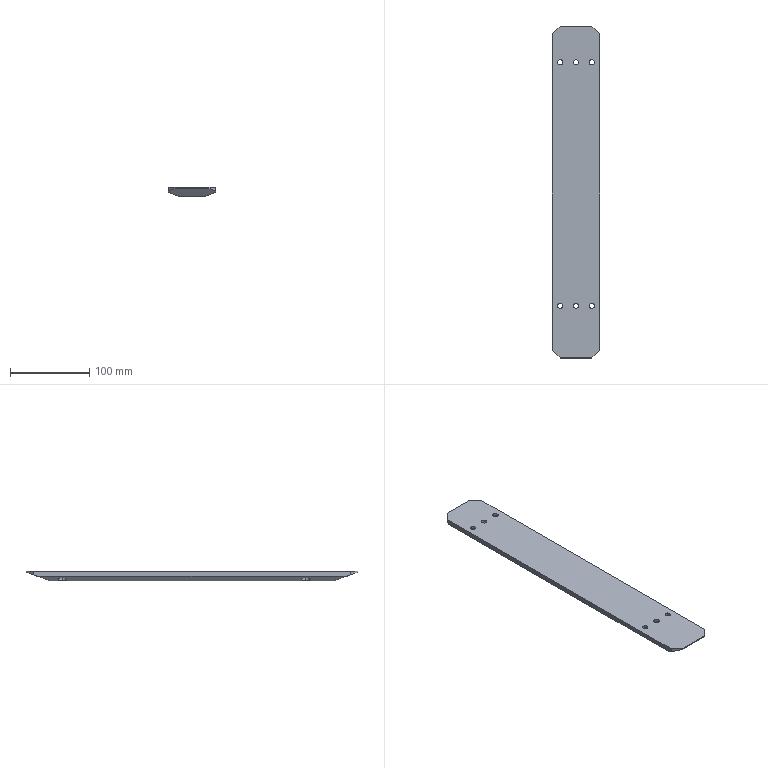Part | SolidWorks | features BaseBody 1 | 1 solid | 44 faces | box 60 x 420 x 12 mm | volume 246931 mm3 | cylinder 24 | plane 20 | commonest cylinder face diameters 6.6 x12 11 x12
STEP:
#1=CARTESIAN_POINT('',(25.5,164.,9.));
#2=VERTEX_POINT('',#1);
#3=CARTESIAN_POINT('',(14.5,164.,9.));
#4=VERTEX_POINT('',#3);
#5=CARTESIAN_POINT('',(20.,164.,9.));
#6=DIRECTION('',(0.,0.,-1.));
#7=DIRECTION('',(-1.,0.,0.));
#8=AXIS2_PLACEMENT_3D('',#5,#6,#7);
#9=CIRCLE('',#8,5.5);
#10=EDGE_CURVE('',#2,#4,#9,.T.);
#11=ORIENTED_EDGE('',*,*,#10,.F.);
#12=CARTESIAN_POINT('',(25.5,164.,3.822));
#13=VERTEX_POINT('',#12);
#14=CARTESIAN_POINT('',(25.5,164.,0.));
#15=DIRECTION('',(0.,0.,-1.));
#16=VECTOR('',#15,1000.);
#17=LINE('',#14,#16);
#18=EDGE_CURVE('',#2,#13,#17,.T.);
#19=ORIENTED_EDGE('',*,*,#18,.T.);
#20=CARTESIAN_POINT('',(15.,161.709,0.));
#21=VERTEX_POINT('',#20);
#22=CARTESIAN_POINT('',(25.5,164.,3.822));
#23=CARTESIAN_POINT('',(25.5,156.466,3.822));
#24=CARTESIAN_POINT('',(18.139,154.859,1.142));
#25=CARTESIAN_POINT('',(15.,161.709,0.));
#26=(BOUNDED_CURVE()B_SPLINE_CURVE(3,(#22,#23,#24,#25),.UNSPECIFIED.,.F.,.F.)B_SPLINE_CURVE_WITH_KNOTS((4,4),(3.142,5.853),.UNSPECIFIED.)CURVE()GEOMETRIC_REPRESENTATION_ITEM()RATIONAL_B_SPLINE_CURVE((1.,0.4755,0.4755,1.))REPRESENTATION_ITEM(''));
#27=EDGE_CURVE('',#13,#21,#26,.T.);
#28=ORIENTED_EDGE('',*,*,#27,.T.);
#29=CARTESIAN_POINT('',(14.5,164.,0.));
#30=VERTEX_POINT('',#29);
#31=CARTESIAN_POINT('',(20.,164.,0.));
#32=DIRECTION('',(0.,0.,-1.));
#33=DIRECTION('',(-1.,0.,0.));
#34=AXIS2_PLACEMENT_3D('',#31,#32,#33);
#35=CIRCLE('',#34,5.5);
#36=EDGE_CURVE('',#21,#30,#35,.T.);
#37=ORIENTED_EDGE('',*,*,#36,.T.);
#38=CARTESIAN_POINT('',(14.5,164.,0.));
#39=DIRECTION('',(0.,0.,-1.));
#40=VECTOR('',#39,1000.);
#41=LINE('',#38,#40);
#42=EDGE_CURVE('',#4,#30,#41,.T.);
#43=ORIENTED_EDGE('',*,*,#42,.F.);
#44=EDGE_LOOP('',(#11,#19,#28,#37,#43));
#45=FACE_OUTER_BOUND('',#44,.T.);
#46=CARTESIAN_POINT('',(20.,164.,0.));
#47=DIRECTION('',(0.,0.,-1.));
#48=DIRECTION('',(-1.,0.,0.));
#49=AXIS2_PLACEMENT_3D('',#46,#47,#48);
#50=CYLINDRICAL_SURFACE('',#49,5.5);
#51=ADVANCED_FACE('',(#45),#50,.F.);
#52=CARTESIAN_POINT('',(23.3,164.,12.));
#53=VERTEX_POINT('',#52);
#54=CARTESIAN_POINT('',(16.7,164.,12.));
#55=VERTEX_POINT('',#54);
#56=CARTESIAN_POINT('',(20.,164.,12.));
#57=DIRECTION('',(0.,0.,-1.));
#58=DIRECTION('',(-1.,0.,0.));
#59=AXIS2_PLACEMENT_3D('',#56,#57,#58);
#60=CIRCLE('',#59,3.3);
#61=EDGE_CURVE('',#53,#55,#60,.T.);
#62=ORIENTED_EDGE('',*,*,#61,.F.);
#63=CARTESIAN_POINT('',(23.3,164.,9.));
#64=VERTEX_POINT('',#63);
#65=CARTESIAN_POINT('',(23.3,164.,0.));
#66=DIRECTION('',(0.,0.,-1.));
#67=VECTOR('',#66,1000.);
#68=LINE('',#65,#67);
#69=EDGE_CURVE('',#53,#64,#68,.T.);
#70=ORIENTED_EDGE('',*,*,#69,.T.);
#71=CARTESIAN_POINT('',(16.7,164.,9.));
#72=VERTEX_POINT('',#71);
#73=CARTESIAN_POINT('',(20.,164.,9.));
#74=DIRECTION('',(0.,0.,-1.));
#75=DIRECTION('',(-1.,0.,0.));
#76=AXIS2_PLACEMENT_3D('',#73,#74,#75);
#77=CIRCLE('',#76,3.3);
#78=EDGE_CURVE('',#64,#72,#77,.T.);
#79=ORIENTED_EDGE('',*,*,#78,.T.);
#80=CARTESIAN_POINT('',(16.7,164.,0.));
#81=DIRECTION('',(0.,0.,-1.));
#82=VECTOR('',#81,1000.);
#83=LINE('',#80,#82);
#84=EDGE_CURVE('',#55,#72,#83,.T.);
#85=ORIENTED_EDGE('',*,*,#84,.F.);
#86=EDGE_LOOP('',(#62,#70,#79,#85));
#87=FACE_OUTER_BOUND('',#86,.T.);
#88=CARTESIAN_POINT('',(20.,164.,0.));
#89=DIRECTION('',(0.,0.,-1.));
#90=DIRECTION('',(-1.,0.,0.));
#91=AXIS2_PLACEMENT_3D('',#88,#89,#90);
#92=CYLINDRICAL_SURFACE('',#91,3.3);
#93=ADVANCED_FACE('',(#87),#92,.F.);
#94=CARTESIAN_POINT('',(5.5,164.,9.));
#95=VERTEX_POINT('',#94);
#96=CARTESIAN_POINT('',(-5.5,164.,9.));
#97=VERTEX_POINT('',#96);
#98=CARTESIAN_POINT('',(0.,164.,9.));
#99=DIRECTION('',(0.,0.,-1.));
#100=DIRECTION('',(-1.,0.,0.));
#101=AXIS2_PLACEMENT_3D('',#98,#99,#100);
#102=CIRCLE('',#101,5.5);
#103=EDGE_CURVE('',#95,#97,#102,.T.);
#104=ORIENTED_EDGE('',*,*,#103,.F.);
#105=CARTESIAN_POINT('',(5.5,164.,0.));
#106=VERTEX_POINT('',#105);
#107=CARTESIAN_POINT('',(5.5,164.,0.));
#108=DIRECTION('',(0.,0.,-1.));
#109=VECTOR('',#108,1000.);
#110=LINE('',#107,#109);
#111=EDGE_CURVE('',#95,#106,#110,.T.);
#112=ORIENTED_EDGE('',*,*,#111,.T.);
#113=CARTESIAN_POINT('',(-5.5,164.,0.));
#114=VERTEX_POINT('',#113);
#115=CARTESIAN_POINT('',(0.,164.,0.));
#116=DIRECTION('',(0.,0.,-1.));
#117=DIRECTION('',(-1.,0.,0.));
#118=AXIS2_PLACEMENT_3D('',#115,#116,#117);
#119=CIRCLE('',#118,5.5);
#120=EDGE_CURVE('',#106,#114,#119,.T.);
#121=ORIENTED_EDGE('',*,*,#120,.T.);
#122=CARTESIAN_POINT('',(-5.5,164.,0.));
#123=DIRECTION('',(0.,0.,-1.));
#124=VECTOR('',#123,1000.);
#125=LINE('',#122,#124);
#126=EDGE_CURVE('',#97,#114,#125,.T.);
#127=ORIENTED_EDGE('',*,*,#126,.F.);
#128=EDGE_LOOP('',(#104,#112,#121,#127));
#129=FACE_OUTER_BOUND('',#128,.T.);
#130=CARTESIAN_POINT('',(0.,164.,0.));
#131=DIRECTION('',(0.,0.,-1.));
#132=DIRECTION('',(-1.,0.,0.));
#133=AXIS2_PLACEMENT_3D('',#130,#131,#132);
#134=CYLINDRICAL_SURFACE('',#133,5.5);
#135=ADVANCED_FACE('',(#129),#134,.F.);
#136=CARTESIAN_POINT('',(3.3,164.,12.));
#137=VERTEX_POINT('',#136);
#138=CARTESIAN_POINT('',(-3.3,164.,12.));
#139=VERTEX_POINT('',#138);
#140=CARTESIAN_POINT('',(0.,164.,12.));
#141=DIRECTION('',(0.,0.,-1.));
#142=DIRECTION('',(-1.,0.,0.));
#143=AXIS2_PLACEMENT_3D('',#140,#141,#142);
#144=CIRCLE('',#143,3.3);
#145=EDGE_CURVE('',#137,#139,#144,.T.);
#146=ORIENTED_EDGE('',*,*,#145,.F.);
#147=CARTESIAN_POINT('',(3.3,164.,9.));
#148=VERTEX_POINT('',#147);
#149=CARTESIAN_POINT('',(3.3,164.,0.));
#150=DIRECTION('',(0.,0.,-1.));
#151=VECTOR('',#150,1000.);
#152=LINE('',#149,#151);
#153=EDGE_CURVE('',#137,#148,#152,.T.);
#154=ORIENTED_EDGE('',*,*,#153,.T.);
#155=CARTESIAN_POINT('',(-3.3,164.,9.));
#156=VERTEX_POINT('',#155);
#157=CARTESIAN_POINT('',(0.,164.,9.));
#158=DIRECTION('',(0.,0.,-1.));
#159=DIRECTION('',(-1.,0.,0.));
#160=AXIS2_PLACEMENT_3D('',#157,#158,#159);
#161=CIRCLE('',#160,3.3);
#162=EDGE_CURVE('',#148,#156,#161,.T.);
#163=ORIENTED_EDGE('',*,*,#162,.T.);
#164=CARTESIAN_POINT('',(-3.3,164.,0.));
#165=DIRECTION('',(0.,0.,-1.));
#166=VECTOR('',#165,1000.);
#167=LINE('',#164,#166);
#168=EDGE_CURVE('',#139,#156,#167,.T.);
#169=ORIENTED_EDGE('',*,*,#168,.F.);
#170=EDGE_LOOP('',(#146,#154,#163,#169));
#171=FACE_OUTER_BOUND('',#170,.T.);
#172=CARTESIAN_POINT('',(0.,164.,0.));
#173=DIRECTION('',(0.,0.,-1.));
#174=DIRECTION('',(-1.,0.,0.));
#175=AXIS2_PLACEMENT_3D('',#172,#173,#174);
#176=CYLINDRICAL_SURFACE('',#175,3.3);
#177=ADVANCED_FACE('',(#171),#176,.F.);
#178=CARTESIAN_POINT('',(-14.5,164.,9.));
#179=VERTEX_POINT('',#178);
#180=CARTESIAN_POINT('',(-25.5,164.,9.));
#181=VERTEX_POINT('',#180);
#182=CARTESIAN_POINT('',(-20.,164.,9.));
#183=DIRECTION('',(0.,0.,-1.));
#184=DIRECTION('',(-1.,0.,0.));
#185=AXIS2_PLACEMENT_3D('',#182,#183,#184);
#186=CIRCLE('',#185,5.5);
#187=EDGE_CURVE('',#179,#181,#186,.T.);
#188=ORIENTED_EDGE('',*,*,#187,.F.);
#189=CARTESIAN_POINT('',(-14.5,164.,0.));
#190=VERTEX_POINT('',#189);
#191=CARTESIAN_POINT('',(-14.5,164.,0.));
#192=DIRECTION('',(0.,0.,-1.));
#193=VECTOR('',#192,1000.);
#194=LINE('',#191,#193);
#195=EDGE_CURVE('',#179,#190,#194,.T.);
#196=ORIENTED_EDGE('',*,*,#195,.T.);
#197=CARTESIAN_POINT('',(-15.,161.709,0.));
#198=VERTEX_POINT('',#197);
#199=CARTESIAN_POINT('',(-20.,164.,0.));
#200=DIRECTION('',(0.,0.,-1.));
#201=DIRECTION('',(-1.,0.,0.));
#202=AXIS2_PLACEMENT_3D('',#199,#200,#201);
#203=CIRCLE('',#202,5.5);
#204=EDGE_CURVE('',#190,#198,#203,.T.);
#205=ORIENTED_EDGE('',*,*,#204,.T.);
#206=CARTESIAN_POINT('',(-25.5,164.,3.822));
#207=VERTEX_POINT('',#206);
#208=CARTESIAN_POINT('',(-15.,161.709,0.));
#209=CARTESIAN_POINT('',(-18.139,154.859,1.142));
#210=CARTESIAN_POINT('',(-25.5,156.466,3.822));
#211=CARTESIAN_POINT('',(-25.5,164.,3.822));
#212=(BOUNDED_CURVE()B_SPLINE_CURVE(3,(#208,#209,#210,#211),.UNSPECIFIED.,.F.,.T.)B_SPLINE_CURVE_WITH_KNOTS((4,4),(0.4297,3.142),.UNSPECIFIED.)CURVE()GEOMETRIC_REPRESENTATION_ITEM()RATIONAL_B_SPLINE_CURVE((1.,0.4755,0.4755,1.))REPRESENTATION_ITEM(''));
#213=EDGE_CURVE('',#198,#207,#212,.T.);
#214=ORIENTED_EDGE('',*,*,#213,.T.);
#215=CARTESIAN_POINT('',(-25.5,164.,0.));
#216=DIRECTION('',(0.,0.,-1.));
#217=VECTOR('',#216,1000.);
#218=LINE('',#215,#217);
#219=EDGE_CURVE('',#181,#207,#218,.T.);
#220=ORIENTED_EDGE('',*,*,#219,.F.);
#221=EDGE_LOOP('',(#188,#196,#205,#214,#220));
#222=FACE_OUTER_BOUND('',#221,.T.);
#223=CARTESIAN_POINT('',(-20.,164.,0.));
#224=DIRECTION('',(0.,0.,-1.));
#225=DIRECTION('',(-1.,0.,0.));
#226=AXIS2_PLACEMENT_3D('',#223,#224,#225);
#227=CYLINDRICAL_SURFACE('',#226,5.5);
#228=ADVANCED_FACE('',(#222),#227,.F.);
#229=CARTESIAN_POINT('',(-16.7,164.,12.));
#230=VERTEX_POINT('',#229);
#231=CARTESIAN_POINT('',(-23.3,164.,12.));
#232=VERTEX_POINT('',#231);
#233=CARTESIAN_POINT('',(-20.,164.,12.));
#234=DIRECTION('',(0.,0.,-1.));
#235=DIRECTION('',(-1.,0.,0.));
#236=AXIS2_PLACEMENT_3D('',#233,#234,#235);
#237=CIRCLE('',#236,3.3);
#238=EDGE_CURVE('',#230,#232,#237,.T.);
#239=ORIENTED_EDGE('',*,*,#238,.F.);
#240=CARTESIAN_POINT('',(-16.7,164.,9.));
#241=VERTEX_POINT('',#240);
#242=CARTESIAN_POINT('',(-16.7,164.,0.));
#243=DIRECTION('',(0.,0.,-1.));
#244=VECTOR('',#243,1000.);
#245=LINE('',#242,#244);
#246=EDGE_CURVE('',#230,#241,#245,.T.);
#247=ORIENTED_EDGE('',*,*,#246,.T.);
#248=CARTESIAN_POINT('',(-23.3,164.,9.));
#249=VERTEX_POINT('',#248);
#250=CARTESIAN_POINT('',(-20.,164.,9.));
#251=DIRECTION('',(0.,0.,-1.));
#252=DIRECTION('',(-1.,0.,0.));
#253=AXIS2_PLACEMENT_3D('',#250,#251,#252);
#254=CIRCLE('',#253,3.3);
#255=EDGE_CURVE('',#241,#249,#254,.T.);
#256=ORIENTED_EDGE('',*,*,#255,.T.);
#257=CARTESIAN_POINT('',(-23.3,164.,0.));
#258=DIRECTION('',(0.,0.,-1.));
#259=VECTOR('',#258,1000.);
#260=LINE('',#257,#259);
#261=EDGE_CURVE('',#232,#249,#260,.T.);
#262=ORIENTED_EDGE('',*,*,#261,.F.);
#263=EDGE_LOOP('',(#239,#247,#256,#262));
#264=FACE_OUTER_BOUND('',#263,.T.);
#265=CARTESIAN_POINT('',(-20.,164.,0.));
#266=DIRECTION('',(0.,0.,-1.));
#267=DIRECTION('',(-1.,0.,0.));
#268=AXIS2_PLACEMENT_3D('',#265,#266,#267);
#269=CYLINDRICAL_SURFACE('',#268,3.3);
#270=ADVANCED_FACE('',(#264),#269,.F.);
#271=CARTESIAN_POINT('',(25.5,-144.,9.));
#272=VERTEX_POINT('',#271);
#273=CARTESIAN_POINT('',(14.5,-144.,9.));
#274=VERTEX_POINT('',#273);
#275=CARTESIAN_POINT('',(20.,-144.,9.));
#276=DIRECTION('',(0.,0.,-1.));
#277=DIRECTION('',(-1.,0.,0.));
#278=AXIS2_PLACEMENT_3D('',#275,#276,#277);
#279=CIRCLE('',#278,5.5);
#280=EDGE_CURVE('',#272,#274,#279,.T.);
#281=ORIENTED_EDGE('',*,*,#280,.F.);
#282=CARTESIAN_POINT('',(25.5,-144.,3.822));
#283=VERTEX_POINT('',#282);
#284=CARTESIAN_POINT('',(25.5,-144.,0.));
#285=DIRECTION('',(0.,0.,-1.));
#286=VECTOR('',#285,1000.);
#287=LINE('',#284,#286);
#288=EDGE_CURVE('',#272,#283,#287,.T.);
#289=ORIENTED_EDGE('',*,*,#288,.T.);
#290=CARTESIAN_POINT('',(15.,-146.291,0.));
#291=VERTEX_POINT('',#290);
#292=CARTESIAN_POINT('',(25.5,-144.,3.822));
#293=CARTESIAN_POINT('',(25.5,-151.534,3.822));
#294=CARTESIAN_POINT('',(18.139,-153.141,1.142));
#295=CARTESIAN_POINT('',(15.,-146.291,0.));
#296=(BOUNDED_CURVE()B_SPLINE_CURVE(3,(#292,#293,#294,#295),.UNSPECIFIED.,.F.,.F.)B_SPLINE_CURVE_WITH_KNOTS((4,4),(3.142,5.853),.UNSPECIFIED.)CURVE()GEOMETRIC_REPRESENTATION_ITEM()RATIONAL_B_SPLINE_CURVE((1.,0.4755,0.4755,1.))REPRESENTATION_ITEM(''));
#297=EDGE_CURVE('',#283,#291,#296,.T.);
#298=ORIENTED_EDGE('',*,*,#297,.T.);
#299=CARTESIAN_POINT('',(14.5,-144.,0.));
#300=VERTEX_POINT('',#299);
#301=CARTESIAN_POINT('',(20.,-144.,0.));
#302=DIRECTION('',(0.,0.,-1.));
#303=DIRECTION('',(-1.,0.,0.));
#304=AXIS2_PLACEMENT_3D('',#301,#302,#303);
#305=CIRCLE('',#304,5.5);
#306=EDGE_CURVE('',#291,#300,#305,.T.);
#307=ORIENTED_EDGE('',*,*,#306,.T.);
#308=CARTESIAN_POINT('',(14.5,-144.,0.));
#309=DIRECTION('',(0.,0.,-1.));
#310=VECTOR('',#309,1000.);
#311=LINE('',#308,#310);
#312=EDGE_CURVE('',#274,#300,#311,.T.);
#313=ORIENTED_EDGE('',*,*,#312,.F.);
#314=EDGE_LOOP('',(#281,#289,#298,#307,#313));
#315=FACE_OUTER_BOUND('',#314,.T.);
#316=CARTESIAN_POINT('',(20.,-144.,0.));
#317=DIRECTION('',(0.,0.,-1.));
#318=DIRECTION('',(-1.,0.,0.));
#319=AXIS2_PLACEMENT_3D('',#316,#317,#318);
#320=CYLINDRICAL_SURFACE('',#319,5.5);
#321=ADVANCED_FACE('',(#315),#320,.F.);
#322=CARTESIAN_POINT('',(23.3,-144.,12.));
#323=VERTEX_POINT('',#322);
#324=CARTESIAN_POINT('',(16.7,-144.,12.));
#325=VERTEX_POINT('',#324);
#326=CARTESIAN_POINT('',(20.,-144.,12.));
#327=DIRECTION('',(0.,0.,-1.));
#328=DIRECTION('',(-1.,0.,0.));
#329=AXIS2_PLACEMENT_3D('',#326,#327,#328);
#330=CIRCLE('',#329,3.3);
#331=EDGE_CURVE('',#323,#325,#330,.T.);
#332=ORIENTED_EDGE('',*,*,#331,.F.);
#333=CARTESIAN_POINT('',(23.3,-144.,9.));
#334=VERTEX_POINT('',#333);
#335=CARTESIAN_POINT('',(23.3,-144.,0.));
#336=DIRECTION('',(0.,0.,-1.));
#337=VECTOR('',#336,1000.);
#338=LINE('',#335,#337);
#339=EDGE_CURVE('',#323,#334,#338,.T.);
#340=ORIENTED_EDGE('',*,*,#339,.T.);
#341=CARTESIAN_POINT('',(16.7,-144.,9.));
#342=VERTEX_POINT('',#341);
#343=CARTESIAN_POINT('',(20.,-144.,9.));
#344=DIRECTION('',(0.,0.,-1.));
#345=DIRECTION('',(-1.,0.,0.));
#346=AXIS2_PLACEMENT_3D('',#343,#344,#345);
#347=CIRCLE('',#346,3.3);
#348=EDGE_CURVE('',#334,#342,#347,.T.);
#349=ORIENTED_EDGE('',*,*,#348,.T.);
#350=CARTESIAN_POINT('',(16.7,-144.,0.));
#351=DIRECTION('',(0.,0.,-1.));
#352=VECTOR('',#351,1000.);
#353=LINE('',#350,#352);
#354=EDGE_CURVE('',#325,#342,#353,.T.);
#355=ORIENTED_EDGE('',*,*,#354,.F.);
#356=EDGE_LOOP('',(#332,#340,#349,#355));
#357=FACE_OUTER_BOUND('',#356,.T.);
#358=CARTESIAN_POINT('',(20.,-144.,0.));
#359=DIRECTION('',(0.,0.,-1.));
#360=DIRECTION('',(-1.,0.,0.));
#361=AXIS2_PLACEMENT_3D('',#358,#359,#360);
#362=CYLINDRICAL_SURFACE('',#361,3.3);
#363=ADVANCED_FACE('',(#357),#362,.F.);
#364=CARTESIAN_POINT('',(5.5,-144.,9.));
#365=VERTEX_POINT('',#364);
#366=CARTESIAN_POINT('',(-5.5,-144.,9.));
#367=VERTEX_POINT('',#366);
#368=CARTESIAN_POINT('',(0.,-144.,9.));
#369=DIRECTION('',(0.,0.,-1.));
#370=DIRECTION('',(-1.,0.,0.));
#371=AXIS2_PLACEMENT_3D('',#368,#369,#370);
#372=CIRCLE('',#371,5.5);
#373=EDGE_CURVE('',#365,#367,#372,.T.);
#374=ORIENTED_EDGE('',*,*,#373,.F.);
#375=CARTESIAN_POINT('',(5.5,-144.,0.));
#376=VERTEX_POINT('',#375);
#377=CARTESIAN_POINT('',(5.5,-144.,0.));
#378=DIRECTION('',(0.,0.,-1.));
#379=VECTOR('',#378,1000.);
#380=LINE('',#377,#379);
#381=EDGE_CURVE('',#365,#376,#380,.T.);
#382=ORIENTED_EDGE('',*,*,#381,.T.);
#383=CARTESIAN_POINT('',(-5.5,-144.,0.));
#384=VERTEX_POINT('',#383);
#385=CARTESIAN_POINT('',(0.,-144.,0.));
#386=DIRECTION('',(0.,0.,-1.));
#387=DIRECTION('',(-1.,0.,0.));
#388=AXIS2_PLACEMENT_3D('',#385,#386,#387);
#389=CIRCLE('',#388,5.5);
#390=EDGE_CURVE('',#376,#384,#389,.T.);
#391=ORIENTED_EDGE('',*,*,#390,.T.);
#392=CARTESIAN_POINT('',(-5.5,-144.,0.));
#393=DIRECTION('',(0.,0.,-1.));
#394=VECTOR('',#393,1000.);
#395=LINE('',#392,#394);
#396=EDGE_CURVE('',#367,#384,#395,.T.);
#397=ORIENTED_EDGE('',*,*,#396,.F.);
#398=EDGE_LOOP('',(#374,#382,#391,#397));
#399=FACE_OUTER_BOUND('',#398,.T.);
#400=CARTESIAN_POINT('',(0.,-144.,0.));
#401=DIRECTION('',(0.,0.,-1.));
#402=DIRECTION('',(-1.,0.,0.));
#403=AXIS2_PLACEMENT_3D('',#400,#401,#402);
#404=CYLINDRICAL_SURFACE('',#403,5.5);
#405=ADVANCED_FACE('',(#399),#404,.F.);
#406=CARTESIAN_POINT('',(3.3,-144.,12.));
#407=VERTEX_POINT('',#406);
#408=CARTESIAN_POINT('',(-3.3,-144.,12.));
#409=VERTEX_POINT('',#408);
#410=CARTESIAN_POINT('',(0.,-144.,12.));
#411=DIRECTION('',(0.,0.,-1.));
#412=DIRECTION('',(-1.,0.,0.));
#413=AXIS2_PLACEMENT_3D('',#410,#411,#412);
#414=CIRCLE('',#413,3.3);
#415=EDGE_CURVE('',#407,#409,#414,.T.);
#416=ORIENTED_EDGE('',*,*,#415,.F.);
#417=CARTESIAN_POINT('',(3.3,-144.,9.));
#418=VERTEX_POINT('',#417);
#419=CARTESIAN_POINT('',(3.3,-144.,0.));
#420=DIRECTION('',(0.,0.,-1.));
#421=VECTOR('',#420,1000.);
#422=LINE('',#419,#421);
#423=EDGE_CURVE('',#407,#418,#422,.T.);
#424=ORIENTED_EDGE('',*,*,#423,.T.);
#425=CARTESIAN_POINT('',(-3.3,-144.,9.));
#426=VERTEX_POINT('',#425);
#427=CARTESIAN_POINT('',(0.,-144.,9.));
#428=DIRECTION('',(0.,0.,-1.));
#429=DIRECTION('',(-1.,0.,0.));
#430=AXIS2_PLACEMENT_3D('',#427,#428,#429);
#431=CIRCLE('',#430,3.3);
#432=EDGE_CURVE('',#418,#426,#431,.T.);
#433=ORIENTED_EDGE('',*,*,#432,.T.);
#434=CARTESIAN_POINT('',(-3.3,-144.,0.));
#435=DIRECTION('',(0.,0.,-1.));
#436=VECTOR('',#435,1000.);
#437=LINE('',#434,#436);
#438=EDGE_CURVE('',#409,#426,#437,.T.);
#439=ORIENTED_EDGE('',*,*,#438,.F.);
#440=EDGE_LOOP('',(#416,#424,#433,#439));
#441=FACE_OUTER_BOUND('',#440,.T.);
#442=CARTESIAN_POINT('',(0.,-144.,0.));
#443=DIRECTION('',(0.,0.,-1.));
#444=DIRECTION('',(-1.,0.,0.));
#445=AXIS2_PLACEMENT_3D('',#442,#443,#444);
#446=CYLINDRICAL_SURFACE('',#445,3.3);
#447=ADVANCED_FACE('',(#441),#446,.F.);
#448=CARTESIAN_POINT('',(-14.5,-144.,9.));
#449=VERTEX_POINT('',#448);
#450=CARTESIAN_POINT('',(-25.5,-144.,9.));
#451=VERTEX_POINT('',#450);
#452=CARTESIAN_POINT('',(-20.,-144.,9.));
#453=DIRECTION('',(0.,0.,-1.));
#454=DIRECTION('',(-1.,0.,0.));
#455=AXIS2_PLACEMENT_3D('',#452,#453,#454);
#456=CIRCLE('',#455,5.5);
#457=EDGE_CURVE('',#449,#451,#456,.T.);
#458=ORIENTED_EDGE('',*,*,#457,.F.);
#459=CARTESIAN_POINT('',(-14.5,-144.,0.));
#460=VERTEX_POINT('',#459);
#461=CARTESIAN_POINT('',(-14.5,-144.,0.));
#462=DIRECTION('',(0.,0.,-1.));
#463=VECTOR('',#462,1000.);
#464=LINE('',#461,#463);
#465=EDGE_CURVE('',#449,#460,#464,.T.);
#466=ORIENTED_EDGE('',*,*,#465,.T.);
#467=CARTESIAN_POINT('',(-15.,-146.291,0.));
#468=VERTEX_POINT('',#467);
#469=CARTESIAN_POINT('',(-20.,-144.,0.));
#470=DIRECTION('',(0.,0.,-1.));
#471=DIRECTION('',(-1.,0.,0.));
#472=AXIS2_PLACEMENT_3D('',#469,#470,#471);
#473=CIRCLE('',#472,5.5);
#474=EDGE_CURVE('',#460,#468,#473,.T.);
#475=ORIENTED_EDGE('',*,*,#474,.T.);
#476=CARTESIAN_POINT('',(-25.5,-144.,3.822));
#477=VERTEX_POINT('',#476);
#478=CARTESIAN_POINT('',(-15.,-146.291,0.));
#479=CARTESIAN_POINT('',(-18.139,-153.141,1.142));
#480=CARTESIAN_POINT('',(-25.5,-151.534,3.822));
#481=CARTESIAN_POINT('',(-25.5,-144.,3.822));
#482=(BOUNDED_CURVE()B_SPLINE_CURVE(3,(#478,#479,#480,#481),.UNSPECIFIED.,.F.,.F.)B_SPLINE_CURVE_WITH_KNOTS((4,4),(0.4297,3.142),.UNSPECIFIED.)CURVE()GEOMETRIC_REPRESENTATION_ITEM()RATIONAL_B_SPLINE_CURVE((1.,0.4755,0.4755,1.))REPRESENTATION_ITEM(''));
#483=EDGE_CURVE('',#468,#477,#482,.T.);
#484=ORIENTED_EDGE('',*,*,#483,.T.);
#485=CARTESIAN_POINT('',(-25.5,-144.,0.));
#486=DIRECTION('',(0.,0.,-1.));
#487=VECTOR('',#486,1000.);
#488=LINE('',#485,#487);
#489=EDGE_CURVE('',#451,#477,#488,.T.);
#490=ORIENTED_EDGE('',*,*,#489,.F.);
#491=EDGE_LOOP('',(#458,#466,#475,#484,#490));
#492=FACE_OUTER_BOUND('',#491,.T.);
#493=CARTESIAN_POINT('',(-20.,-144.,0.));
#494=DIRECTION('',(0.,0.,-1.));
#495=DIRECTION('',(-1.,0.,0.));
#496=AXIS2_PLACEMENT_3D('',#493,#494,#495);
#497=CYLINDRICAL_SURFACE('',#496,5.5);
#498=ADVANCED_FACE('',(#492),#497,.F.);
#499=CARTESIAN_POINT('',(-16.7,-144.,12.));
#500=VERTEX_POINT('',#499);
#501=CARTESIAN_POINT('',(-23.3,-144.,12.));
#502=VERTEX_POINT('',#501);
#503=CARTESIAN_POINT('',(-20.,-144.,12.));
#504=DIRECTION('',(0.,0.,-1.));
#505=DIRECTION('',(-1.,0.,0.));
#506=AXIS2_PLACEMENT_3D('',#503,#504,#505);
#507=CIRCLE('',#506,3.3);
#508=EDGE_CURVE('',#500,#502,#507,.T.);
#509=ORIENTED_EDGE('',*,*,#508,.F.);
#510=CARTESIAN_POINT('',(-16.7,-144.,9.));
#511=VERTEX_POINT('',#510);
#512=CARTESIAN_POINT('',(-16.7,-144.,0.));
#513=DIRECTION('',(0.,0.,-1.));
#514=VECTOR('',#513,1000.);
#515=LINE('',#512,#514);
#516=EDGE_CURVE('',#500,#511,#515,.T.);
#517=ORIENTED_EDGE('',*,*,#516,.T.);
#518=CARTESIAN_POINT('',(-23.3,-144.,9.));
#519=VERTEX_POINT('',#518);
#520=CARTESIAN_POINT('',(-20.,-144.,9.));
#521=DIRECTION('',(0.,0.,-1.));
#522=DIRECTION('',(-1.,0.,0.));
#523=AXIS2_PLACEMENT_3D('',#520,#521,#522);
#524=CIRCLE('',#523,3.3);
#525=EDGE_CURVE('',#511,#519,#524,.T.);
#526=ORIENTED_EDGE('',*,*,#525,.T.);
#527=CARTESIAN_POINT('',(-23.3,-144.,0.));
#528=DIRECTION('',(0.,0.,-1.));
#529=VECTOR('',#528,1000.);
#530=LINE('',#527,#529);
#531=EDGE_CURVE('',#502,#519,#530,.T.);
#532=ORIENTED_EDGE('',*,*,#531,.F.);
#533=EDGE_LOOP('',(#509,#517,#526,#532));
#534=FACE_OUTER_BOUND('',#533,.T.);
#535=CARTESIAN_POINT('',(-20.,-144.,0.));
#536=DIRECTION('',(0.,0.,-1.));
#537=DIRECTION('',(-1.,0.,0.));
#538=AXIS2_PLACEMENT_3D('',#535,#536,#537);
#539=CYLINDRICAL_SURFACE('',#538,3.3);
#540=ADVANCED_FACE('',(#534),#539,.F.);
#541=CARTESIAN_POINT('',(20.,164.,12.));
#542=DIRECTION('',(0.,0.,-1.));
#543=DIRECTION('',(-1.,0.,0.));
#544=AXIS2_PLACEMENT_3D('',#541,#542,#543);
#545=CIRCLE('',#544,3.3);
#546=EDGE_CURVE('',#55,#53,#545,.T.);
#547=ORIENTED_EDGE('',*,*,#546,.T.);
#548=ORIENTED_EDGE('',*,*,#61,.T.);
#549=EDGE_LOOP('',(#547,#548));
#550=FACE_BOUND('',#549,.T.);
#551=CARTESIAN_POINT('',(0.,164.,12.));
#552=DIRECTION('',(0.,0.,-1.));
#553=DIRECTION('',(-1.,0.,0.));
#554=AXIS2_PLACEMENT_3D('',#551,#552,#553);
#555=CIRCLE('',#554,3.3);
#556=EDGE_CURVE('',#139,#137,#555,.T.);
#557=ORIENTED_EDGE('',*,*,#556,.T.);
#558=ORIENTED_EDGE('',*,*,#145,.T.);
#559=EDGE_LOOP('',(#557,#558));
#560=FACE_BOUND('',#559,.T.);
#561=CARTESIAN_POINT('',(-20.,-210.,12.));
#562=VERTEX_POINT('',#561);
#563=CARTESIAN_POINT('',(20.,-210.,12.));
#564=VERTEX_POINT('',#563);
#565=CARTESIAN_POINT('',(-30.,-210.,12.));
#566=DIRECTION('',(1.,0.,0.));
#567=VECTOR('',#566,1000.);
#568=LINE('',#565,#567);
#569=EDGE_CURVE('',#562,#564,#568,.T.);
#570=ORIENTED_EDGE('',*,*,#569,.T.);
#571=CARTESIAN_POINT('',(30.,-200.,12.));
#572=VERTEX_POINT('',#571);
#573=CARTESIAN_POINT('',(115.,-115.,12.));
#574=DIRECTION('',(0.7071,0.7071,0.));
#575=VECTOR('',#574,1000.);
#576=LINE('',#573,#575);
#577=EDGE_CURVE('',#564,#572,#576,.T.);
#578=ORIENTED_EDGE('',*,*,#577,.T.);
#579=CARTESIAN_POINT('',(30.,200.,12.));
#580=VERTEX_POINT('',#579);
#581=CARTESIAN_POINT('',(30.,210.,12.));
#582=DIRECTION('',(0.,1.,0.));
#583=VECTOR('',#582,1000.);
#584=LINE('',#581,#583);
#585=EDGE_CURVE('',#572,#580,#584,.T.);
#586=ORIENTED_EDGE('',*,*,#585,.T.);
#587=CARTESIAN_POINT('',(20.,210.,12.));
#588=VERTEX_POINT('',#587);
#589=CARTESIAN_POINT('',(115.,115.,12.));
#590=DIRECTION('',(-0.7071,0.7071,0.));
#591=VECTOR('',#590,1000.);
#592=LINE('',#589,#591);
#593=EDGE_CURVE('',#580,#588,#592,.T.);
#594=ORIENTED_EDGE('',*,*,#593,.T.);
#595=CARTESIAN_POINT('',(-20.,210.,12.));
#596=VERTEX_POINT('',#595);
#597=CARTESIAN_POINT('',(-30.,210.,12.));
#598=DIRECTION('',(-1.,0.,0.));
#599=VECTOR('',#598,1000.);
#600=LINE('',#597,#599);
#601=EDGE_CURVE('',#588,#596,#600,.T.);
#602=ORIENTED_EDGE('',*,*,#601,.T.);
#603=CARTESIAN_POINT('',(-30.,200.,12.));
#604=VERTEX_POINT('',#603);
#605=CARTESIAN_POINT('',(-115.,115.,12.));
#606=DIRECTION('',(-0.7071,-0.7071,0.));
#607=VECTOR('',#606,1000.);
#608=LINE('',#605,#607);
#609=EDGE_CURVE('',#596,#604,#608,.T.);
#610=ORIENTED_EDGE('',*,*,#609,.T.);
#611=CARTESIAN_POINT('',(-30.,-200.,12.));
#612=VERTEX_POINT('',#611);
#613=CARTESIAN_POINT('',(-30.,210.,12.));
#614=DIRECTION('',(0.,-1.,0.));
#615=VECTOR('',#614,1000.);
#616=LINE('',#613,#615);
#617=EDGE_CURVE('',#604,#612,#616,.T.);
#618=ORIENTED_EDGE('',*,*,#617,.T.);
#619=CARTESIAN_POINT('',(-115.,-115.,12.));
#620=DIRECTION('',(0.7071,-0.7071,0.));
#621=VECTOR('',#620,1000.);
#622=LINE('',#619,#621);
#623=EDGE_CURVE('',#612,#562,#622,.T.);
#624=ORIENTED_EDGE('',*,*,#623,.T.);
#625=EDGE_LOOP('',(#570,#578,#586,#594,#602,#610,#618,#624));
#626=FACE_OUTER_BOUND('',#625,.T.);
#627=CARTESIAN_POINT('',(-20.,-144.,12.));
#628=DIRECTION('',(0.,0.,-1.));
#629=DIRECTION('',(-1.,0.,0.));
#630=AXIS2_PLACEMENT_3D('',#627,#628,#629);
#631=CIRCLE('',#630,3.3);
#632=EDGE_CURVE('',#502,#500,#631,.T.);
#633=ORIENTED_EDGE('',*,*,#632,.T.);
#634=ORIENTED_EDGE('',*,*,#508,.T.);
#635=EDGE_LOOP('',(#633,#634));
#636=FACE_BOUND('',#635,.T.);
#637=CARTESIAN_POINT('',(0.,-144.,12.));
#638=DIRECTION('',(0.,0.,-1.));
#639=DIRECTION('',(-1.,0.,0.));
#640=AXIS2_PLACEMENT_3D('',#637,#638,#639);
#641=CIRCLE('',#640,3.3);
#642=EDGE_CURVE('',#409,#407,#641,.T.);
#643=ORIENTED_EDGE('',*,*,#642,.T.);
#644=ORIENTED_EDGE('',*,*,#415,.T.);
#645=EDGE_LOOP('',(#643,#644));
#646=FACE_BOUND('',#645,.T.);
#647=CARTESIAN_POINT('',(20.,-144.,12.));
#648=DIRECTION('',(0.,0.,-1.));
#649=DIRECTION('',(-1.,0.,0.));
#650=AXIS2_PLACEMENT_3D('',#647,#648,#649);
#651=CIRCLE('',#650,3.3);
#652=EDGE_CURVE('',#325,#323,#651,.T.);
#653=ORIENTED_EDGE('',*,*,#652,.T.);
#654=ORIENTED_EDGE('',*,*,#331,.T.);
#655=EDGE_LOOP('',(#653,#654));
#656=FACE_BOUND('',#655,.T.);
#657=CARTESIAN_POINT('',(-20.,164.,12.));
#658=DIRECTION('',(0.,0.,-1.));
#659=DIRECTION('',(-1.,0.,0.));
#660=AXIS2_PLACEMENT_3D('',#657,#658,#659);
#661=CIRCLE('',#660,3.3);
#662=EDGE_CURVE('',#232,#230,#661,.T.);
#663=ORIENTED_EDGE('',*,*,#662,.T.);
#664=ORIENTED_EDGE('',*,*,#238,.T.);
#665=EDGE_LOOP('',(#663,#664));
#666=FACE_BOUND('',#665,.T.);
#667=CARTESIAN_POINT('',(0.,0.,12.));
#668=DIRECTION('',(0.,0.,1.));
#669=DIRECTION('',(1.,0.,0.));
#670=AXIS2_PLACEMENT_3D('',#667,#668,#669);
#671=PLANE('',#670);
#672=ADVANCED_FACE('',(#550,#560,#626,#636,#646,#656,#666),#671,.T.);
#673=CARTESIAN_POINT('',(0.,164.,0.));
#674=DIRECTION('',(0.,0.,-1.));
#675=DIRECTION('',(-1.,0.,0.));
#676=AXIS2_PLACEMENT_3D('',#673,#674,#675);
#677=CIRCLE('',#676,5.5);
#678=EDGE_CURVE('',#114,#106,#677,.T.);
#679=ORIENTED_EDGE('',*,*,#678,.F.);
#680=ORIENTED_EDGE('',*,*,#120,.F.);
#681=EDGE_LOOP('',(#679,#680));
#682=FACE_BOUND('',#681,.T.);
#683=CARTESIAN_POINT('',(0.,-144.,0.));
#684=DIRECTION('',(0.,0.,-1.));
#685=DIRECTION('',(-1.,0.,0.));
#686=AXIS2_PLACEMENT_3D('',#683,#684,#685);
#687=CIRCLE('',#686,5.5);
#688=EDGE_CURVE('',#384,#376,#687,.T.);
#689=ORIENTED_EDGE('',*,*,#688,.F.);
#690=ORIENTED_EDGE('',*,*,#390,.F.);
#691=EDGE_LOOP('',(#689,#690));
#692=FACE_BOUND('',#691,.T.);
#693=CARTESIAN_POINT('',(15.,180.,0.));
#694=VERTEX_POINT('',#693);
#695=CARTESIAN_POINT('',(15.,166.291,0.));
#696=VERTEX_POINT('',#695);
#697=CARTESIAN_POINT('',(15.,0.,0.));
#698=DIRECTION('',(0.,-1.,0.));
#699=VECTOR('',#698,1000.);
#700=LINE('',#697,#699);
#701=EDGE_CURVE('',#694,#696,#700,.T.);
#702=ORIENTED_EDGE('',*,*,#701,.T.);
#703=CARTESIAN_POINT('',(20.,164.,0.));
#704=DIRECTION('',(0.,0.,-1.));
#705=DIRECTION('',(-1.,0.,0.));
#706=AXIS2_PLACEMENT_3D('',#703,#704,#705);
#707=CIRCLE('',#706,5.5);
#708=EDGE_CURVE('',#30,#696,#707,.T.);
#709=ORIENTED_EDGE('',*,*,#708,.F.);
#710=ORIENTED_EDGE('',*,*,#36,.F.);
#711=CARTESIAN_POINT('',(15.,-141.709,0.));
#712=VERTEX_POINT('',#711);
#713=CARTESIAN_POINT('',(15.,0.,0.));
#714=DIRECTION('',(0.,-1.,0.));
#715=VECTOR('',#714,1000.);
#716=LINE('',#713,#715);
#717=EDGE_CURVE('',#21,#712,#716,.T.);
#718=ORIENTED_EDGE('',*,*,#717,.T.);
#719=CARTESIAN_POINT('',(20.,-144.,0.));
#720=DIRECTION('',(0.,0.,-1.));
#721=DIRECTION('',(-1.,0.,0.));
#722=AXIS2_PLACEMENT_3D('',#719,#720,#721);
#723=CIRCLE('',#722,5.5);
#724=EDGE_CURVE('',#300,#712,#723,.T.);
#725=ORIENTED_EDGE('',*,*,#724,.F.);
#726=ORIENTED_EDGE('',*,*,#306,.F.);
#727=CARTESIAN_POINT('',(15.,-180.,0.));
#728=VERTEX_POINT('',#727);
#729=CARTESIAN_POINT('',(15.,0.,0.));
#730=DIRECTION('',(0.,-1.,0.));
#731=VECTOR('',#730,1000.);
#732=LINE('',#729,#731);
#733=EDGE_CURVE('',#291,#728,#732,.T.);
#734=ORIENTED_EDGE('',*,*,#733,.T.);
#735=CARTESIAN_POINT('',(-15.,-180.,0.));
#736=VERTEX_POINT('',#735);
#737=CARTESIAN_POINT('',(0.,-180.,0.));
#738=DIRECTION('',(-1.,0.,0.));
#739=VECTOR('',#738,1000.);
#740=LINE('',#737,#739);
#741=EDGE_CURVE('',#728,#736,#740,.T.);
#742=ORIENTED_EDGE('',*,*,#741,.T.);
#743=CARTESIAN_POINT('',(-15.,0.,0.));
#744=DIRECTION('',(0.,1.,0.));
#745=VECTOR('',#744,1000.);
#746=LINE('',#743,#745);
#747=EDGE_CURVE('',#736,#468,#746,.T.);
#748=ORIENTED_EDGE('',*,*,#747,.T.);
#749=ORIENTED_EDGE('',*,*,#474,.F.);
#750=CARTESIAN_POINT('',(-15.,-141.709,0.));
#751=VERTEX_POINT('',#750);
#752=CARTESIAN_POINT('',(-20.,-144.,0.));
#753=DIRECTION('',(0.,0.,-1.));
#754=DIRECTION('',(-1.,0.,0.));
#755=AXIS2_PLACEMENT_3D('',#752,#753,#754);
#756=CIRCLE('',#755,5.5);
#757=EDGE_CURVE('',#751,#460,#756,.T.);
#758=ORIENTED_EDGE('',*,*,#757,.F.);
#759=CARTESIAN_POINT('',(-15.,0.,0.));
#760=DIRECTION('',(0.,1.,0.));
#761=VECTOR('',#760,1000.);
#762=LINE('',#759,#761);
#763=EDGE_CURVE('',#751,#198,#762,.T.);
#764=ORIENTED_EDGE('',*,*,#763,.T.);
#765=ORIENTED_EDGE('',*,*,#204,.F.);
#766=CARTESIAN_POINT('',(-15.,166.291,0.));
#767=VERTEX_POINT('',#766);
#768=CARTESIAN_POINT('',(-20.,164.,0.));
#769=DIRECTION('',(0.,0.,-1.));
#770=DIRECTION('',(-1.,0.,0.));
#771=AXIS2_PLACEMENT_3D('',#768,#769,#770);
#772=CIRCLE('',#771,5.5);
#773=EDGE_CURVE('',#767,#190,#772,.T.);
#774=ORIENTED_EDGE('',*,*,#773,.F.);
#775=CARTESIAN_POINT('',(-15.,180.,0.));
#776=VERTEX_POINT('',#775);
#777=CARTESIAN_POINT('',(-15.,0.,0.));
#778=DIRECTION('',(0.,1.,0.));
#779=VECTOR('',#778,1000.);
#780=LINE('',#777,#779);
#781=EDGE_CURVE('',#767,#776,#780,.T.);
#782=ORIENTED_EDGE('',*,*,#781,.T.);
#783=CARTESIAN_POINT('',(0.,180.,0.));
#784=DIRECTION('',(1.,0.,0.));
#785=VECTOR('',#784,1000.);
#786=LINE('',#783,#785);
#787=EDGE_CURVE('',#776,#694,#786,.T.);
#788=ORIENTED_EDGE('',*,*,#787,.T.);
#789=EDGE_LOOP('',(#702,#709,#710,#718,#725,#726,#734,#742,#748,#749,#758,#764,#765,#774,#782,#788));
#790=FACE_OUTER_BOUND('',#789,.T.);
#791=CARTESIAN_POINT('',(0.,0.,0.));
#792=DIRECTION('',(0.,0.,1.));
#793=DIRECTION('',(1.,0.,0.));
#794=AXIS2_PLACEMENT_3D('',#791,#792,#793);
#795=PLANE('',#794);
#796=ADVANCED_FACE('',(#682,#692,#790),#795,.F.);
#797=CARTESIAN_POINT('',(30.,-200.,7.279));
#798=VERTEX_POINT('',#797);
#799=CARTESIAN_POINT('',(30.,-195.,5.46));
#800=VERTEX_POINT('',#799);
#801=CARTESIAN_POINT('',(30.,-210.,10.919));
#802=DIRECTION('',(0.,0.9397,-0.342));
#803=VECTOR('',#802,1000.);
#804=LINE('',#801,#803);
#805=EDGE_CURVE('',#798,#800,#804,.T.);
#806=ORIENTED_EDGE('',*,*,#805,.T.);
#807=CARTESIAN_POINT('',(30.,195.,5.46));
#808=VERTEX_POINT('',#807);
#809=CARTESIAN_POINT('',(30.,210.,5.46));
#810=DIRECTION('',(0.,1.,0.));
#811=VECTOR('',#810,1000.);
#812=LINE('',#809,#811);
#813=EDGE_CURVE('',#800,#808,#812,.T.);
#814=ORIENTED_EDGE('',*,*,#813,.T.);
#815=CARTESIAN_POINT('',(30.,200.,7.279));
#816=VERTEX_POINT('',#815);
#817=CARTESIAN_POINT('',(30.,210.,10.919));
#818=DIRECTION('',(0.,0.9397,0.342));
#819=VECTOR('',#818,1000.);
#820=LINE('',#817,#819);
#821=EDGE_CURVE('',#808,#816,#820,.T.);
#822=ORIENTED_EDGE('',*,*,#821,.T.);
#823=CARTESIAN_POINT('',(30.,200.,12.));
#824=DIRECTION('',(0.,0.,1.));
#825=VECTOR('',#824,1000.);
#826=LINE('',#823,#825);
#827=EDGE_CURVE('',#816,#580,#826,.T.);
#828=ORIENTED_EDGE('',*,*,#827,.T.);
#829=ORIENTED_EDGE('',*,*,#585,.F.);
#830=CARTESIAN_POINT('',(30.,-200.,12.));
#831=DIRECTION('',(0.,0.,-1.));
#832=VECTOR('',#831,1000.);
#833=LINE('',#830,#832);
#834=EDGE_CURVE('',#572,#798,#833,.T.);
#835=ORIENTED_EDGE('',*,*,#834,.T.);
#836=EDGE_LOOP('',(#806,#814,#822,#828,#829,#835));
#837=FACE_OUTER_BOUND('',#836,.T.);
#838=CARTESIAN_POINT('',(30.,210.,12.));
#839=DIRECTION('',(-1.,0.,0.));
#840=DIRECTION('',(0.,-1.,0.));
#841=AXIS2_PLACEMENT_3D('',#838,#839,#840);
#842=PLANE('',#841);
#843=ADVANCED_FACE('',(#837),#842,.F.);
#844=CARTESIAN_POINT('',(20.,210.,10.919));
#845=VERTEX_POINT('',#844);
#846=CARTESIAN_POINT('',(20.,210.,12.));
#847=DIRECTION('',(0.,0.,-1.));
#848=VECTOR('',#847,1000.);
#849=LINE('',#846,#848);
#850=EDGE_CURVE('',#588,#845,#849,.T.);
#851=ORIENTED_EDGE('',*,*,#850,.T.);
#852=CARTESIAN_POINT('',(-20.,210.,10.919));
#853=VERTEX_POINT('',#852);
#854=CARTESIAN_POINT('',(-30.,210.,10.919));
#855=DIRECTION('',(-1.,0.,0.));
#856=VECTOR('',#855,1000.);
#857=LINE('',#854,#856);
#858=EDGE_CURVE('',#845,#853,#857,.T.);
#859=ORIENTED_EDGE('',*,*,#858,.T.);
#860=CARTESIAN_POINT('',(-20.,210.,12.));
#861=DIRECTION('',(0.,0.,1.));
#862=VECTOR('',#861,1000.);
#863=LINE('',#860,#862);
#864=EDGE_CURVE('',#853,#596,#863,.T.);
#865=ORIENTED_EDGE('',*,*,#864,.T.);
#866=ORIENTED_EDGE('',*,*,#601,.F.);
#867=EDGE_LOOP('',(#851,#859,#865,#866));
#868=FACE_OUTER_BOUND('',#867,.T.);
#869=CARTESIAN_POINT('',(-30.,210.,12.));
#870=DIRECTION('',(0.,-1.,0.));
#871=DIRECTION('',(0.,0.,-1.));
#872=AXIS2_PLACEMENT_3D('',#869,#870,#871);
#873=PLANE('',#872);
#874=ADVANCED_FACE('',(#868),#873,.F.);
#875=CARTESIAN_POINT('',(-30.,200.,7.279));
#876=VERTEX_POINT('',#875);
#877=CARTESIAN_POINT('',(-30.,195.,5.46));
#878=VERTEX_POINT('',#877);
#879=CARTESIAN_POINT('',(-30.,210.,10.919));
#880=DIRECTION('',(0.,-0.9397,-0.342));
#881=VECTOR('',#880,1000.);
#882=LINE('',#879,#881);
#883=EDGE_CURVE('',#876,#878,#882,.T.);
#884=ORIENTED_EDGE('',*,*,#883,.T.);
#885=CARTESIAN_POINT('',(-30.,-195.,5.46));
#886=VERTEX_POINT('',#885);
#887=CARTESIAN_POINT('',(-30.,210.,5.46));
#888=DIRECTION('',(0.,-1.,0.));
#889=VECTOR('',#888,1000.);
#890=LINE('',#887,#889);
#891=EDGE_CURVE('',#878,#886,#890,.T.);
#892=ORIENTED_EDGE('',*,*,#891,.T.);
#893=CARTESIAN_POINT('',(-30.,-200.,7.279));
#894=VERTEX_POINT('',#893);
#895=CARTESIAN_POINT('',(-30.,-210.,10.919));
#896=DIRECTION('',(0.,-0.9397,0.342));
#897=VECTOR('',#896,1000.);
#898=LINE('',#895,#897);
#899=EDGE_CURVE('',#886,#894,#898,.T.);
#900=ORIENTED_EDGE('',*,*,#899,.T.);
#901=CARTESIAN_POINT('',(-30.,-200.,12.));
#902=DIRECTION('',(0.,0.,1.));
#903=VECTOR('',#902,1000.);
#904=LINE('',#901,#903);
#905=EDGE_CURVE('',#894,#612,#904,.T.);
#906=ORIENTED_EDGE('',*,*,#905,.T.);
#907=ORIENTED_EDGE('',*,*,#617,.F.);
#908=CARTESIAN_POINT('',(-30.,200.,12.));
#909=DIRECTION('',(0.,0.,-1.));
#910=VECTOR('',#909,1000.);
#911=LINE('',#908,#910);
#912=EDGE_CURVE('',#604,#876,#911,.T.);
#913=ORIENTED_EDGE('',*,*,#912,.T.);
#914=EDGE_LOOP('',(#884,#892,#900,#906,#907,#913));
#915=FACE_OUTER_BOUND('',#914,.T.);
#916=CARTESIAN_POINT('',(-30.,210.,12.));
#917=DIRECTION('',(1.,0.,0.));
#918=DIRECTION('',(0.,1.,0.));
#919=AXIS2_PLACEMENT_3D('',#916,#917,#918);
#920=PLANE('',#919);
#921=ADVANCED_FACE('',(#915),#920,.F.);
#922=CARTESIAN_POINT('',(-20.,-210.,10.919));
#923=VERTEX_POINT('',#922);
#924=CARTESIAN_POINT('',(-20.,-210.,12.));
#925=DIRECTION('',(0.,0.,-1.));
#926=VECTOR('',#925,1000.);
#927=LINE('',#924,#926);
#928=EDGE_CURVE('',#562,#923,#927,.T.);
#929=ORIENTED_EDGE('',*,*,#928,.T.);
#930=CARTESIAN_POINT('',(20.,-210.,10.919));
#931=VERTEX_POINT('',#930);
#932=CARTESIAN_POINT('',(-30.,-210.,10.919));
#933=DIRECTION('',(1.,0.,0.));
#934=VECTOR('',#933,1000.);
#935=LINE('',#932,#934);
#936=EDGE_CURVE('',#923,#931,#935,.T.);
#937=ORIENTED_EDGE('',*,*,#936,.T.);
#938=CARTESIAN_POINT('',(20.,-210.,12.));
#939=DIRECTION('',(0.,0.,1.));
#940=VECTOR('',#939,1000.);
#941=LINE('',#938,#940);
#942=EDGE_CURVE('',#931,#564,#941,.T.);
#943=ORIENTED_EDGE('',*,*,#942,.T.);
#944=ORIENTED_EDGE('',*,*,#569,.F.);
#945=EDGE_LOOP('',(#929,#937,#943,#944));
#946=FACE_OUTER_BOUND('',#945,.T.);
#947=CARTESIAN_POINT('',(-30.,-210.,12.));
#948=DIRECTION('',(0.,1.,0.));
#949=DIRECTION('',(0.,0.,1.));
#950=AXIS2_PLACEMENT_3D('',#947,#948,#949);
#951=PLANE('',#950);
#952=ADVANCED_FACE('',(#946),#951,.F.);
#953=ORIENTED_EDGE('',*,*,#942,.F.);
#954=CARTESIAN_POINT('',(29.194,-200.806,7.573));
#955=DIRECTION('',(0.6848,0.6848,-0.2492));
#956=VECTOR('',#955,1000.);
#957=LINE('',#954,#956);
#958=EDGE_CURVE('',#931,#798,#957,.T.);
#959=ORIENTED_EDGE('',*,*,#958,.T.);
#960=ORIENTED_EDGE('',*,*,#834,.F.);
#961=ORIENTED_EDGE('',*,*,#577,.F.);
#962=EDGE_LOOP('',(#953,#959,#960,#961));
#963=FACE_OUTER_BOUND('',#962,.T.);
#964=CARTESIAN_POINT('',(30.,-200.,12.));
#965=DIRECTION('',(-0.7071,0.7071,0.));
#966=DIRECTION('',(0.,0.,-1.));
#967=AXIS2_PLACEMENT_3D('',#964,#965,#966);
#968=PLANE('',#967);
#969=ADVANCED_FACE('',(#963),#968,.F.);
#970=ORIENTED_EDGE('',*,*,#905,.F.);
#971=CARTESIAN_POINT('',(-19.816,-210.184,10.986));
#972=DIRECTION('',(0.6848,-0.6848,0.2492));
#973=VECTOR('',#972,1000.);
#974=LINE('',#971,#973);
#975=EDGE_CURVE('',#894,#923,#974,.T.);
#976=ORIENTED_EDGE('',*,*,#975,.T.);
#977=ORIENTED_EDGE('',*,*,#928,.F.);
#978=ORIENTED_EDGE('',*,*,#623,.F.);
#979=EDGE_LOOP('',(#970,#976,#977,#978));
#980=FACE_OUTER_BOUND('',#979,.T.);
#981=CARTESIAN_POINT('',(-20.,-210.,12.));
#982=DIRECTION('',(0.7071,0.7071,0.));
#983=DIRECTION('',(0.,0.,-1.));
#984=AXIS2_PLACEMENT_3D('',#981,#982,#983);
#985=PLANE('',#984);
#986=ADVANCED_FACE('',(#980),#985,.F.);
#987=ORIENTED_EDGE('',*,*,#827,.F.);
#988=CARTESIAN_POINT('',(19.816,210.184,10.986));
#989=DIRECTION('',(-0.6848,0.6848,0.2492));
#990=VECTOR('',#989,1000.);
#991=LINE('',#988,#990);
#992=EDGE_CURVE('',#816,#845,#991,.T.);
#993=ORIENTED_EDGE('',*,*,#992,.T.);
#994=ORIENTED_EDGE('',*,*,#850,.F.);
#995=ORIENTED_EDGE('',*,*,#593,.F.);
#996=EDGE_LOOP('',(#987,#993,#994,#995));
#997=FACE_OUTER_BOUND('',#996,.T.);
#998=CARTESIAN_POINT('',(20.,210.,12.));
#999=DIRECTION('',(-0.7071,-0.7071,0.));
#1000=DIRECTION('',(0.,0.,-1.));
#1001=AXIS2_PLACEMENT_3D('',#998,#999,#1000);
#1002=PLANE('',#1001);
#1003=ADVANCED_FACE('',(#997),#1002,.F.);
#1004=ORIENTED_EDGE('',*,*,#864,.F.);
#1005=CARTESIAN_POINT('',(-29.194,200.806,7.573));
#1006=DIRECTION('',(-0.6848,-0.6848,-0.2492));
#1007=VECTOR('',#1006,1000.);
#1008=LINE('',#1005,#1007);
#1009=EDGE_CURVE('',#853,#876,#1008,.T.);
#1010=ORIENTED_EDGE('',*,*,#1009,.T.);
#1011=ORIENTED_EDGE('',*,*,#912,.F.);
#1012=ORIENTED_EDGE('',*,*,#609,.F.);
#1013=EDGE_LOOP('',(#1004,#1010,#1011,#1012));
#1014=FACE_OUTER_BOUND('',#1013,.T.);
#1015=CARTESIAN_POINT('',(-30.,200.,12.));
#1016=DIRECTION('',(0.7071,-0.7071,0.));
#1017=DIRECTION('',(0.,0.,-1.));
#1018=AXIS2_PLACEMENT_3D('',#1015,#1016,#1017);
#1019=PLANE('',#1018);
#1020=ADVANCED_FACE('',(#1014),#1019,.F.);
#1021=ORIENTED_EDGE('',*,*,#787,.F.);
#1022=CARTESIAN_POINT('',(-37.966,202.966,8.359));
#1023=DIRECTION('',(-0.6848,0.6848,0.2492));
#1024=VECTOR('',#1023,1000.);
#1025=LINE('',#1022,#1024);
#1026=EDGE_CURVE('',#776,#878,#1025,.T.);
#1027=ORIENTED_EDGE('',*,*,#1026,.T.);
#1028=ORIENTED_EDGE('',*,*,#883,.F.);
#1029=ORIENTED_EDGE('',*,*,#1009,.F.);
#1030=ORIENTED_EDGE('',*,*,#858,.F.);
#1031=ORIENTED_EDGE('',*,*,#992,.F.);
#1032=ORIENTED_EDGE('',*,*,#821,.F.);
#1033=CARTESIAN_POINT('',(9.83,174.83,-1.882));
#1034=DIRECTION('',(-0.6848,-0.6848,-0.2492));
#1035=VECTOR('',#1034,1000.);
#1036=LINE('',#1033,#1035);
#1037=EDGE_CURVE('',#808,#694,#1036,.T.);
#1038=ORIENTED_EDGE('',*,*,#1037,.T.);
#1039=EDGE_LOOP('',(#1021,#1027,#1028,#1029,#1030,#1031,#1032,#1038));
#1040=FACE_OUTER_BOUND('',#1039,.T.);
#1041=CARTESIAN_POINT('',(-30.,210.,10.919));
#1042=DIRECTION('',(0.,-0.342,0.9397));
#1043=DIRECTION('',(-1.,0.,0.));
#1044=AXIS2_PLACEMENT_3D('',#1041,#1042,#1043);
#1045=PLANE('',#1044);
#1046=ADVANCED_FACE('',(#1040),#1045,.F.);
#1047=ORIENTED_EDGE('',*,*,#899,.F.);
#1048=CARTESIAN_POINT('',(-37.966,-202.966,8.359));
#1049=DIRECTION('',(0.6848,0.6848,-0.2492));
#1050=VECTOR('',#1049,1000.);
#1051=LINE('',#1048,#1050);
#1052=EDGE_CURVE('',#886,#736,#1051,.T.);
#1053=ORIENTED_EDGE('',*,*,#1052,.T.);
#1054=ORIENTED_EDGE('',*,*,#741,.F.);
#1055=CARTESIAN_POINT('',(9.83,-174.83,-1.882));
#1056=DIRECTION('',(0.6848,-0.6848,0.2492));
#1057=VECTOR('',#1056,1000.);
#1058=LINE('',#1055,#1057);
#1059=EDGE_CURVE('',#728,#800,#1058,.T.);
#1060=ORIENTED_EDGE('',*,*,#1059,.T.);
#1061=ORIENTED_EDGE('',*,*,#805,.F.);
#1062=ORIENTED_EDGE('',*,*,#958,.F.);
#1063=ORIENTED_EDGE('',*,*,#936,.F.);
#1064=ORIENTED_EDGE('',*,*,#975,.F.);
#1065=EDGE_LOOP('',(#1047,#1053,#1054,#1060,#1061,#1062,#1063,#1064));
#1066=FACE_OUTER_BOUND('',#1065,.T.);
#1067=CARTESIAN_POINT('',(-30.,-210.,10.919));
#1068=DIRECTION('',(0.,0.342,0.9397));
#1069=DIRECTION('',(1.,0.,0.));
#1070=AXIS2_PLACEMENT_3D('',#1067,#1068,#1069);
#1071=PLANE('',#1070);
#1072=ADVANCED_FACE('',(#1066),#1071,.F.);
#1073=ORIENTED_EDGE('',*,*,#213,.F.);
#1074=ORIENTED_EDGE('',*,*,#763,.F.);
#1075=CARTESIAN_POINT('',(-25.5,-144.,3.822));
#1076=CARTESIAN_POINT('',(-25.5,-136.466,3.822));
#1077=CARTESIAN_POINT('',(-18.139,-134.859,1.142));
#1078=CARTESIAN_POINT('',(-15.,-141.709,0.));
#1079=(BOUNDED_CURVE()B_SPLINE_CURVE(3,(#1075,#1076,#1077,#1078),.UNSPECIFIED.,.F.,.F.)B_SPLINE_CURVE_WITH_KNOTS((4,4),(3.142,5.853),.UNSPECIFIED.)CURVE()GEOMETRIC_REPRESENTATION_ITEM()RATIONAL_B_SPLINE_CURVE((1.,0.4755,0.4755,1.))REPRESENTATION_ITEM(''));
#1080=EDGE_CURVE('',#477,#751,#1079,.T.);
#1081=ORIENTED_EDGE('',*,*,#1080,.F.);
#1082=ORIENTED_EDGE('',*,*,#483,.F.);
#1083=ORIENTED_EDGE('',*,*,#747,.F.);
#1084=ORIENTED_EDGE('',*,*,#1052,.F.);
#1085=ORIENTED_EDGE('',*,*,#891,.F.);
#1086=ORIENTED_EDGE('',*,*,#1026,.F.);
#1087=ORIENTED_EDGE('',*,*,#781,.F.);
#1088=CARTESIAN_POINT('',(-25.5,164.,3.822));
#1089=CARTESIAN_POINT('',(-25.5,171.534,3.822));
#1090=CARTESIAN_POINT('',(-18.139,173.141,1.142));
#1091=CARTESIAN_POINT('',(-15.,166.291,0.));
#1092=(BOUNDED_CURVE()B_SPLINE_CURVE(3,(#1088,#1089,#1090,#1091),.UNSPECIFIED.,.F.,.F.)B_SPLINE_CURVE_WITH_KNOTS((4,4),(3.142,5.853),.UNSPECIFIED.)CURVE()GEOMETRIC_REPRESENTATION_ITEM()RATIONAL_B_SPLINE_CURVE((1.,0.4755,0.4755,1.))REPRESENTATION_ITEM(''));
#1093=EDGE_CURVE('',#207,#767,#1092,.T.);
#1094=ORIENTED_EDGE('',*,*,#1093,.F.);
#1095=EDGE_LOOP('',(#1073,#1074,#1081,#1082,#1083,#1084,#1085,#1086,#1087,#1094));
#1096=FACE_OUTER_BOUND('',#1095,.T.);
#1097=CARTESIAN_POINT('',(-30.,210.,5.46));
#1098=DIRECTION('',(0.342,0.,0.9397));
#1099=DIRECTION('',(0.,-1.,0.));
#1100=AXIS2_PLACEMENT_3D('',#1097,#1098,#1099);
#1101=PLANE('',#1100);
#1102=ADVANCED_FACE('',(#1096),#1101,.F.);
#1103=CARTESIAN_POINT('',(15.,166.291,0.));
#1104=CARTESIAN_POINT('',(18.139,173.141,1.142));
#1105=CARTESIAN_POINT('',(25.5,171.534,3.822));
#1106=CARTESIAN_POINT('',(25.5,164.,3.822));
#1107=(BOUNDED_CURVE()B_SPLINE_CURVE(3,(#1103,#1104,#1105,#1106),.UNSPECIFIED.,.F.,.F.)B_SPLINE_CURVE_WITH_KNOTS((4,4),(0.4297,3.142),.UNSPECIFIED.)CURVE()GEOMETRIC_REPRESENTATION_ITEM()RATIONAL_B_SPLINE_CURVE((1.,0.4755,0.4755,1.))REPRESENTATION_ITEM(''));
#1108=EDGE_CURVE('',#696,#13,#1107,.T.);
#1109=ORIENTED_EDGE('',*,*,#1108,.F.);
#1110=ORIENTED_EDGE('',*,*,#701,.F.);
#1111=ORIENTED_EDGE('',*,*,#1037,.F.);
#1112=ORIENTED_EDGE('',*,*,#813,.F.);
#1113=ORIENTED_EDGE('',*,*,#1059,.F.);
#1114=ORIENTED_EDGE('',*,*,#733,.F.);
#1115=ORIENTED_EDGE('',*,*,#297,.F.);
#1116=CARTESIAN_POINT('',(15.,-141.709,0.));
#1117=CARTESIAN_POINT('',(18.139,-134.859,1.142));
#1118=CARTESIAN_POINT('',(25.5,-136.466,3.822));
#1119=CARTESIAN_POINT('',(25.5,-144.,3.822));
#1120=(BOUNDED_CURVE()B_SPLINE_CURVE(3,(#1116,#1117,#1118,#1119),.UNSPECIFIED.,.F.,.F.)B_SPLINE_CURVE_WITH_KNOTS((4,4),(0.4297,3.142),.UNSPECIFIED.)CURVE()GEOMETRIC_REPRESENTATION_ITEM()RATIONAL_B_SPLINE_CURVE((1.,0.4755,0.4755,1.))REPRESENTATION_ITEM(''));
#1121=EDGE_CURVE('',#712,#283,#1120,.T.);
#1122=ORIENTED_EDGE('',*,*,#1121,.F.);
#1123=ORIENTED_EDGE('',*,*,#717,.F.);
#1124=ORIENTED_EDGE('',*,*,#27,.F.);
#1125=EDGE_LOOP('',(#1109,#1110,#1111,#1112,#1113,#1114,#1115,#1122,#1123,#1124));
#1126=FACE_OUTER_BOUND('',#1125,.T.);
#1127=CARTESIAN_POINT('',(30.,210.,5.46));
#1128=DIRECTION('',(-0.342,0.,0.9397));
#1129=DIRECTION('',(0.,1.,0.));
#1130=AXIS2_PLACEMENT_3D('',#1127,#1128,#1129);
#1131=PLANE('',#1130);
#1132=ADVANCED_FACE('',(#1126),#1131,.F.);
#1133=ORIENTED_EDGE('',*,*,#516,.F.);
#1134=ORIENTED_EDGE('',*,*,#632,.F.);
#1135=ORIENTED_EDGE('',*,*,#531,.T.);
#1136=CARTESIAN_POINT('',(-20.,-144.,9.));
#1137=DIRECTION('',(0.,0.,-1.));
#1138=DIRECTION('',(-1.,0.,0.));
#1139=AXIS2_PLACEMENT_3D('',#1136,#1137,#1138);
#1140=CIRCLE('',#1139,3.3);
#1141=EDGE_CURVE('',#519,#511,#1140,.T.);
#1142=ORIENTED_EDGE('',*,*,#1141,.T.);
#1143=EDGE_LOOP('',(#1133,#1134,#1135,#1142));
#1144=FACE_OUTER_BOUND('',#1143,.T.);
#1145=CARTESIAN_POINT('',(-20.,-144.,0.));
#1146=DIRECTION('',(0.,0.,-1.));
#1147=DIRECTION('',(-1.,0.,0.));
#1148=AXIS2_PLACEMENT_3D('',#1145,#1146,#1147);
#1149=CYLINDRICAL_SURFACE('',#1148,3.3);
#1150=ADVANCED_FACE('',(#1144),#1149,.F.);
#1151=ORIENTED_EDGE('',*,*,#1141,.F.);
#1152=ORIENTED_EDGE('',*,*,#525,.F.);
#1153=EDGE_LOOP('',(#1151,#1152));
#1154=FACE_BOUND('',#1153,.T.);
#1155=CARTESIAN_POINT('',(-20.,-144.,9.));
#1156=DIRECTION('',(0.,0.,-1.));
#1157=DIRECTION('',(-1.,0.,0.));
#1158=AXIS2_PLACEMENT_3D('',#1155,#1156,#1157);
#1159=CIRCLE('',#1158,5.5);
#1160=EDGE_CURVE('',#451,#449,#1159,.T.);
#1161=ORIENTED_EDGE('',*,*,#1160,.T.);
#1162=ORIENTED_EDGE('',*,*,#457,.T.);
#1163=EDGE_LOOP('',(#1161,#1162));
#1164=FACE_OUTER_BOUND('',#1163,.T.);
#1165=CARTESIAN_POINT('',(-16.7,-144.,9.));
#1166=DIRECTION('',(0.,0.,1.));
#1167=DIRECTION('',(1.,0.,0.));
#1168=AXIS2_PLACEMENT_3D('',#1165,#1166,#1167);
#1169=PLANE('',#1168);
#1170=ADVANCED_FACE('',(#1154,#1164),#1169,.F.);
#1171=ORIENTED_EDGE('',*,*,#465,.F.);
#1172=ORIENTED_EDGE('',*,*,#1160,.F.);
#1173=ORIENTED_EDGE('',*,*,#489,.T.);
#1174=ORIENTED_EDGE('',*,*,#1080,.T.);
#1175=ORIENTED_EDGE('',*,*,#757,.T.);
#1176=EDGE_LOOP('',(#1171,#1172,#1173,#1174,#1175));
#1177=FACE_OUTER_BOUND('',#1176,.T.);
#1178=CARTESIAN_POINT('',(-20.,-144.,0.));
#1179=DIRECTION('',(0.,0.,-1.));
#1180=DIRECTION('',(-1.,0.,0.));
#1181=AXIS2_PLACEMENT_3D('',#1178,#1179,#1180);
#1182=CYLINDRICAL_SURFACE('',#1181,5.5);
#1183=ADVANCED_FACE('',(#1177),#1182,.F.);
#1184=ORIENTED_EDGE('',*,*,#423,.F.);
#1185=ORIENTED_EDGE('',*,*,#642,.F.);
#1186=ORIENTED_EDGE('',*,*,#438,.T.);
#1187=CARTESIAN_POINT('',(0.,-144.,9.));
#1188=DIRECTION('',(0.,0.,-1.));
#1189=DIRECTION('',(-1.,0.,0.));
#1190=AXIS2_PLACEMENT_3D('',#1187,#1188,#1189);
#1191=CIRCLE('',#1190,3.3);
#1192=EDGE_CURVE('',#426,#418,#1191,.T.);
#1193=ORIENTED_EDGE('',*,*,#1192,.T.);
#1194=EDGE_LOOP('',(#1184,#1185,#1186,#1193));
#1195=FACE_OUTER_BOUND('',#1194,.T.);
#1196=CARTESIAN_POINT('',(0.,-144.,0.));
#1197=DIRECTION('',(0.,0.,-1.));
#1198=DIRECTION('',(-1.,0.,0.));
#1199=AXIS2_PLACEMENT_3D('',#1196,#1197,#1198);
#1200=CYLINDRICAL_SURFACE('',#1199,3.3);
#1201=ADVANCED_FACE('',(#1195),#1200,.F.);
#1202=ORIENTED_EDGE('',*,*,#1192,.F.);
#1203=ORIENTED_EDGE('',*,*,#432,.F.);
#1204=EDGE_LOOP('',(#1202,#1203));
#1205=FACE_BOUND('',#1204,.T.);
#1206=CARTESIAN_POINT('',(0.,-144.,9.));
#1207=DIRECTION('',(0.,0.,-1.));
#1208=DIRECTION('',(-1.,0.,0.));
#1209=AXIS2_PLACEMENT_3D('',#1206,#1207,#1208);
#1210=CIRCLE('',#1209,5.5);
#1211=EDGE_CURVE('',#367,#365,#1210,.T.);
#1212=ORIENTED_EDGE('',*,*,#1211,.T.);
#1213=ORIENTED_EDGE('',*,*,#373,.T.);
#1214=EDGE_LOOP('',(#1212,#1213));
#1215=FACE_OUTER_BOUND('',#1214,.T.);
#1216=CARTESIAN_POINT('',(3.3,-144.,9.));
#1217=DIRECTION('',(0.,0.,1.));
#1218=DIRECTION('',(1.,0.,0.));
#1219=AXIS2_PLACEMENT_3D('',#1216,#1217,#1218);
#1220=PLANE('',#1219);
#1221=ADVANCED_FACE('',(#1205,#1215),#1220,.F.);
#1222=ORIENTED_EDGE('',*,*,#381,.F.);
#1223=ORIENTED_EDGE('',*,*,#1211,.F.);
#1224=ORIENTED_EDGE('',*,*,#396,.T.);
#1225=ORIENTED_EDGE('',*,*,#688,.T.);
#1226=EDGE_LOOP('',(#1222,#1223,#1224,#1225));
#1227=FACE_OUTER_BOUND('',#1226,.T.);
#1228=CARTESIAN_POINT('',(0.,-144.,0.));
#1229=DIRECTION('',(0.,0.,-1.));
#1230=DIRECTION('',(-1.,0.,0.));
#1231=AXIS2_PLACEMENT_3D('',#1228,#1229,#1230);
#1232=CYLINDRICAL_SURFACE('',#1231,5.5);
#1233=ADVANCED_FACE('',(#1227),#1232,.F.);
#1234=ORIENTED_EDGE('',*,*,#339,.F.);
#1235=ORIENTED_EDGE('',*,*,#652,.F.);
#1236=ORIENTED_EDGE('',*,*,#354,.T.);
#1237=CARTESIAN_POINT('',(20.,-144.,9.));
#1238=DIRECTION('',(0.,0.,-1.));
#1239=DIRECTION('',(-1.,0.,0.));
#1240=AXIS2_PLACEMENT_3D('',#1237,#1238,#1239);
#1241=CIRCLE('',#1240,3.3);
#1242=EDGE_CURVE('',#342,#334,#1241,.T.);
#1243=ORIENTED_EDGE('',*,*,#1242,.T.);
#1244=EDGE_LOOP('',(#1234,#1235,#1236,#1243));
#1245=FACE_OUTER_BOUND('',#1244,.T.);
#1246=CARTESIAN_POINT('',(20.,-144.,0.));
#1247=DIRECTION('',(0.,0.,-1.));
#1248=DIRECTION('',(-1.,0.,0.));
#1249=AXIS2_PLACEMENT_3D('',#1246,#1247,#1248);
#1250=CYLINDRICAL_SURFACE('',#1249,3.3);
#1251=ADVANCED_FACE('',(#1245),#1250,.F.);
#1252=ORIENTED_EDGE('',*,*,#1242,.F.);
#1253=ORIENTED_EDGE('',*,*,#348,.F.);
#1254=EDGE_LOOP('',(#1252,#1253));
#1255=FACE_BOUND('',#1254,.T.);
#1256=CARTESIAN_POINT('',(20.,-144.,9.));
#1257=DIRECTION('',(0.,0.,-1.));
#1258=DIRECTION('',(-1.,0.,0.));
#1259=AXIS2_PLACEMENT_3D('',#1256,#1257,#1258);
#1260=CIRCLE('',#1259,5.5);
#1261=EDGE_CURVE('',#274,#272,#1260,.T.);
#1262=ORIENTED_EDGE('',*,*,#1261,.T.);
#1263=ORIENTED_EDGE('',*,*,#280,.T.);
#1264=EDGE_LOOP('',(#1262,#1263));
#1265=FACE_OUTER_BOUND('',#1264,.T.);
#1266=CARTESIAN_POINT('',(23.3,-144.,9.));
#1267=DIRECTION('',(0.,0.,1.));
#1268=DIRECTION('',(1.,0.,0.));
#1269=AXIS2_PLACEMENT_3D('',#1266,#1267,#1268);
#1270=PLANE('',#1269);
#1271=ADVANCED_FACE('',(#1255,#1265),#1270,.F.);
#1272=ORIENTED_EDGE('',*,*,#288,.F.);
#1273=ORIENTED_EDGE('',*,*,#1261,.F.);
#1274=ORIENTED_EDGE('',*,*,#312,.T.);
#1275=ORIENTED_EDGE('',*,*,#724,.T.);
#1276=ORIENTED_EDGE('',*,*,#1121,.T.);
#1277=EDGE_LOOP('',(#1272,#1273,#1274,#1275,#1276));
#1278=FACE_OUTER_BOUND('',#1277,.T.);
#1279=CARTESIAN_POINT('',(20.,-144.,0.));
#1280=DIRECTION('',(0.,0.,-1.));
#1281=DIRECTION('',(-1.,0.,0.));
#1282=AXIS2_PLACEMENT_3D('',#1279,#1280,#1281);
#1283=CYLINDRICAL_SURFACE('',#1282,5.5);
#1284=ADVANCED_FACE('',(#1278),#1283,.F.);
#1285=ORIENTED_EDGE('',*,*,#246,.F.);
#1286=ORIENTED_EDGE('',*,*,#662,.F.);
#1287=ORIENTED_EDGE('',*,*,#261,.T.);
#1288=CARTESIAN_POINT('',(-20.,164.,9.));
#1289=DIRECTION('',(0.,0.,-1.));
#1290=DIRECTION('',(-1.,0.,0.));
#1291=AXIS2_PLACEMENT_3D('',#1288,#1289,#1290);
#1292=CIRCLE('',#1291,3.3);
#1293=EDGE_CURVE('',#249,#241,#1292,.T.);
#1294=ORIENTED_EDGE('',*,*,#1293,.T.);
#1295=EDGE_LOOP('',(#1285,#1286,#1287,#1294));
#1296=FACE_OUTER_BOUND('',#1295,.T.);
#1297=CARTESIAN_POINT('',(-20.,164.,0.));
#1298=DIRECTION('',(0.,0.,-1.));
#1299=DIRECTION('',(-1.,0.,0.));
#1300=AXIS2_PLACEMENT_3D('',#1297,#1298,#1299);
#1301=CYLINDRICAL_SURFACE('',#1300,3.3);
#1302=ADVANCED_FACE('',(#1296),#1301,.F.);
#1303=ORIENTED_EDGE('',*,*,#1293,.F.);
#1304=ORIENTED_EDGE('',*,*,#255,.F.);
#1305=EDGE_LOOP('',(#1303,#1304));
#1306=FACE_BOUND('',#1305,.T.);
#1307=CARTESIAN_POINT('',(-20.,164.,9.));
#1308=DIRECTION('',(0.,0.,-1.));
#1309=DIRECTION('',(-1.,0.,0.));
#1310=AXIS2_PLACEMENT_3D('',#1307,#1308,#1309);
#1311=CIRCLE('',#1310,5.5);
#1312=EDGE_CURVE('',#181,#179,#1311,.T.);
#1313=ORIENTED_EDGE('',*,*,#1312,.T.);
#1314=ORIENTED_EDGE('',*,*,#187,.T.);
#1315=EDGE_LOOP('',(#1313,#1314));
#1316=FACE_OUTER_BOUND('',#1315,.T.);
#1317=CARTESIAN_POINT('',(-16.7,164.,9.));
#1318=DIRECTION('',(0.,0.,1.));
#1319=DIRECTION('',(1.,0.,0.));
#1320=AXIS2_PLACEMENT_3D('',#1317,#1318,#1319);
#1321=PLANE('',#1320);
#1322=ADVANCED_FACE('',(#1306,#1316),#1321,.F.);
#1323=ORIENTED_EDGE('',*,*,#195,.F.);
#1324=ORIENTED_EDGE('',*,*,#1312,.F.);
#1325=ORIENTED_EDGE('',*,*,#219,.T.);
#1326=ORIENTED_EDGE('',*,*,#1093,.T.);
#1327=ORIENTED_EDGE('',*,*,#773,.T.);
#1328=EDGE_LOOP('',(#1323,#1324,#1325,#1326,#1327));
#1329=FACE_OUTER_BOUND('',#1328,.T.);
#1330=CARTESIAN_POINT('',(-20.,164.,0.));
#1331=DIRECTION('',(0.,0.,-1.));
#1332=DIRECTION('',(-1.,0.,0.));
#1333=AXIS2_PLACEMENT_3D('',#1330,#1331,#1332);
#1334=CYLINDRICAL_SURFACE('',#1333,5.5);
#1335=ADVANCED_FACE('',(#1329),#1334,.F.);
#1336=ORIENTED_EDGE('',*,*,#153,.F.);
#1337=ORIENTED_EDGE('',*,*,#556,.F.);
#1338=ORIENTED_EDGE('',*,*,#168,.T.);
#1339=CARTESIAN_POINT('',(0.,164.,9.));
#1340=DIRECTION('',(0.,0.,-1.));
#1341=DIRECTION('',(-1.,0.,0.));
#1342=AXIS2_PLACEMENT_3D('',#1339,#1340,#1341);
#1343=CIRCLE('',#1342,3.3);
#1344=EDGE_CURVE('',#156,#148,#1343,.T.);
#1345=ORIENTED_EDGE('',*,*,#1344,.T.);
#1346=EDGE_LOOP('',(#1336,#1337,#1338,#1345));
#1347=FACE_OUTER_BOUND('',#1346,.T.);
#1348=CARTESIAN_POINT('',(0.,164.,0.));
#1349=DIRECTION('',(0.,0.,-1.));
#1350=DIRECTION('',(-1.,0.,0.));
#1351=AXIS2_PLACEMENT_3D('',#1348,#1349,#1350);
#1352=CYLINDRICAL_SURFACE('',#1351,3.3);
#1353=ADVANCED_FACE('',(#1347),#1352,.F.);
#1354=ORIENTED_EDGE('',*,*,#1344,.F.);
#1355=ORIENTED_EDGE('',*,*,#162,.F.);
#1356=EDGE_LOOP('',(#1354,#1355));
#1357=FACE_BOUND('',#1356,.T.);
#1358=CARTESIAN_POINT('',(0.,164.,9.));
#1359=DIRECTION('',(0.,0.,-1.));
#1360=DIRECTION('',(-1.,0.,0.));
#1361=AXIS2_PLACEMENT_3D('',#1358,#1359,#1360);
#1362=CIRCLE('',#1361,5.5);
#1363=EDGE_CURVE('',#97,#95,#1362,.T.);
#1364=ORIENTED_EDGE('',*,*,#1363,.T.);
#1365=ORIENTED_EDGE('',*,*,#103,.T.);
#1366=EDGE_LOOP('',(#1364,#1365));
#1367=FACE_OUTER_BOUND('',#1366,.T.);
#1368=CARTESIAN_POINT('',(3.3,164.,9.));
#1369=DIRECTION('',(0.,0.,1.));
#1370=DIRECTION('',(1.,0.,0.));
#1371=AXIS2_PLACEMENT_3D('',#1368,#1369,#1370);
#1372=PLANE('',#1371);
#1373=ADVANCED_FACE('',(#1357,#1367),#1372,.F.);
#1374=ORIENTED_EDGE('',*,*,#111,.F.);
#1375=ORIENTED_EDGE('',*,*,#1363,.F.);
#1376=ORIENTED_EDGE('',*,*,#126,.T.);
#1377=ORIENTED_EDGE('',*,*,#678,.T.);
#1378=EDGE_LOOP('',(#1374,#1375,#1376,#1377));
#1379=FACE_OUTER_BOUND('',#1378,.T.);
#1380=CARTESIAN_POINT('',(0.,164.,0.));
#1381=DIRECTION('',(0.,0.,-1.));
#1382=DIRECTION('',(-1.,0.,0.));
#1383=AXIS2_PLACEMENT_3D('',#1380,#1381,#1382);
#1384=CYLINDRICAL_SURFACE('',#1383,5.5);
#1385=ADVANCED_FACE('',(#1379),#1384,.F.);
#1386=ORIENTED_EDGE('',*,*,#69,.F.);
#1387=ORIENTED_EDGE('',*,*,#546,.F.);
#1388=ORIENTED_EDGE('',*,*,#84,.T.);
#1389=CARTESIAN_POINT('',(20.,164.,9.));
#1390=DIRECTION('',(0.,0.,-1.));
#1391=DIRECTION('',(-1.,0.,0.));
#1392=AXIS2_PLACEMENT_3D('',#1389,#1390,#1391);
#1393=CIRCLE('',#1392,3.3);
#1394=EDGE_CURVE('',#72,#64,#1393,.T.);
#1395=ORIENTED_EDGE('',*,*,#1394,.T.);
#1396=EDGE_LOOP('',(#1386,#1387,#1388,#1395));
#1397=FACE_OUTER_BOUND('',#1396,.T.);
#1398=CARTESIAN_POINT('',(20.,164.,0.));
#1399=DIRECTION('',(0.,0.,-1.));
#1400=DIRECTION('',(-1.,0.,0.));
#1401=AXIS2_PLACEMENT_3D('',#1398,#1399,#1400);
#1402=CYLINDRICAL_SURFACE('',#1401,3.3);
#1403=ADVANCED_FACE('',(#1397),#1402,.F.);
#1404=ORIENTED_EDGE('',*,*,#1394,.F.);
#1405=ORIENTED_EDGE('',*,*,#78,.F.);
#1406=EDGE_LOOP('',(#1404,#1405));
#1407=FACE_BOUND('',#1406,.T.);
#1408=CARTESIAN_POINT('',(20.,164.,9.));
#1409=DIRECTION('',(0.,0.,-1.));
#1410=DIRECTION('',(-1.,0.,0.));
#1411=AXIS2_PLACEMENT_3D('',#1408,#1409,#1410);
#1412=CIRCLE('',#1411,5.5);
#1413=EDGE_CURVE('',#4,#2,#1412,.T.);
#1414=ORIENTED_EDGE('',*,*,#1413,.T.);
#1415=ORIENTED_EDGE('',*,*,#10,.T.);
#1416=EDGE_LOOP('',(#1414,#1415));
#1417=FACE_OUTER_BOUND('',#1416,.T.);
#1418=CARTESIAN_POINT('',(23.3,164.,9.));
#1419=DIRECTION('',(0.,0.,1.));
#1420=DIRECTION('',(1.,0.,0.));
#1421=AXIS2_PLACEMENT_3D('',#1418,#1419,#1420);
#1422=PLANE('',#1421);
#1423=ADVANCED_FACE('',(#1407,#1417),#1422,.F.);
#1424=ORIENTED_EDGE('',*,*,#18,.F.);
#1425=ORIENTED_EDGE('',*,*,#1413,.F.);
#1426=ORIENTED_EDGE('',*,*,#42,.T.);
#1427=ORIENTED_EDGE('',*,*,#708,.T.);
#1428=ORIENTED_EDGE('',*,*,#1108,.T.);
#1429=EDGE_LOOP('',(#1424,#1425,#1426,#1427,#1428));
#1430=FACE_OUTER_BOUND('',#1429,.T.);
#1431=CARTESIAN_POINT('',(20.,164.,0.));
#1432=DIRECTION('',(0.,0.,-1.));
#1433=DIRECTION('',(-1.,0.,0.));
#1434=AXIS2_PLACEMENT_3D('',#1431,#1432,#1433);
#1435=CYLINDRICAL_SURFACE('',#1434,5.5);
#1436=ADVANCED_FACE('',(#1430),#1435,.F.);
#1437=CLOSED_SHELL('',(#51,#93,#135,#177,#228,#270,#321,#363,#405,#447,#498,#540,#672,#796,#843,#874,#921,#952,#969,#986,#1003,#1020,#1046,#1072,#1102,#1132,#1150,#1170,#1183,#1201,#1221,#1233,#1251,#1271,#1284,#1302,#1322,#1335,#1353,#1373,#1385,#1403,#1423,#1436));
#1438=MANIFOLD_SOLID_BREP('',#1437);
#1439=CARTESIAN_POINT('',(0.,0.,0.));
#1440=DIRECTION('',(0.,0.,1.));
#1441=DIRECTION('',(1.,0.,0.));
#1442=AXIS2_PLACEMENT_3D('',#1439,#1440,#1441);
#1443=(LENGTH_UNIT()NAMED_UNIT(*)SI_UNIT(.MILLI.,.METRE.));
#1444=UNCERTAINTY_MEASURE_WITH_UNIT(LENGTH_MEASURE(0.00001),#1443,'','');
#1445=(NAMED_UNIT(*)PLANE_ANGLE_UNIT()SI_UNIT($,.RADIAN.));
#1446=(NAMED_UNIT(*)SI_UNIT($,.STERADIAN.)SOLID_ANGLE_UNIT());
#1447=(GEOMETRIC_REPRESENTATION_CONTEXT(3)GLOBAL_UNCERTAINTY_ASSIGNED_CONTEXT((#1444))GLOBAL_UNIT_ASSIGNED_CONTEXT((#1443,#1445,#1446))REPRESENTATION_CONTEXT('',''));
#1448=ADVANCED_BREP_SHAPE_REPRESENTATION('',(#1438,#1442),#1447);